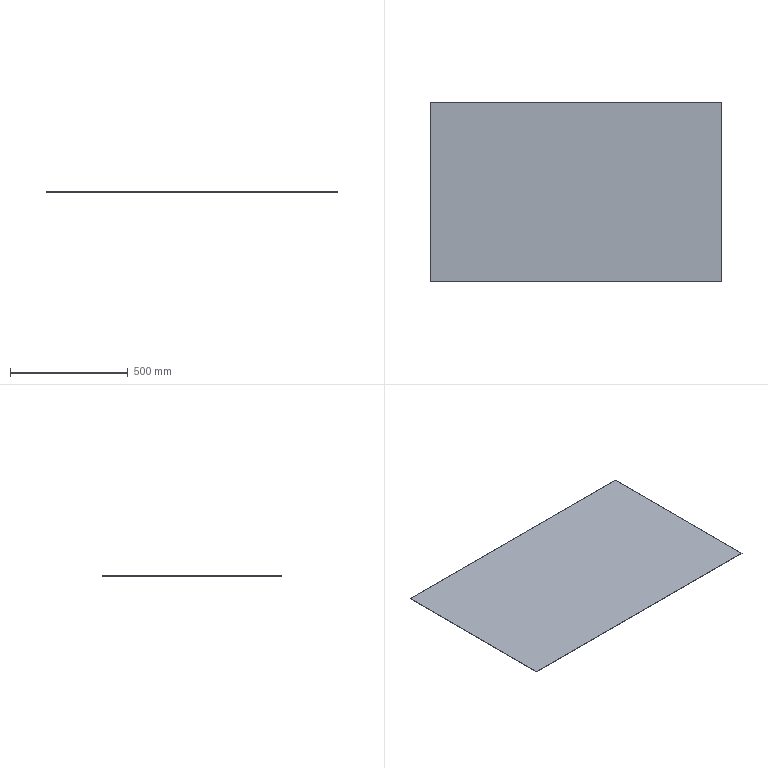Part | SolidWorks | 1 solid | 6 faces | box 1230 x 760 x 1.5 mm | volume 1402200 mm3 | plane 6
STEP:
#1=CARTESIAN_POINT('',(615.,-380.,0.));
#2=VERTEX_POINT('',#1);
#3=CARTESIAN_POINT('',(615.,380.,0.));
#4=VERTEX_POINT('',#3);
#5=CARTESIAN_POINT('',(615.,-380.,0.));
#6=DIRECTION('',(0.,1.,0.));
#7=VECTOR('',#6,1000.);
#8=LINE('',#5,#7);
#9=EDGE_CURVE('',#2,#4,#8,.T.);
#10=ORIENTED_EDGE('',*,*,#9,.T.);
#11=CARTESIAN_POINT('',(615.,380.,1.5));
#12=VERTEX_POINT('',#11);
#13=CARTESIAN_POINT('',(615.,380.,1.5));
#14=DIRECTION('',(0.,0.,-1.));
#15=VECTOR('',#14,1000.);
#16=LINE('',#13,#15);
#17=EDGE_CURVE('',#12,#4,#16,.T.);
#18=ORIENTED_EDGE('',*,*,#17,.F.);
#19=CARTESIAN_POINT('',(615.,-380.,1.5));
#20=VERTEX_POINT('',#19);
#21=CARTESIAN_POINT('',(615.,-380.,1.5));
#22=DIRECTION('',(0.,1.,0.));
#23=VECTOR('',#22,1000.);
#24=LINE('',#21,#23);
#25=EDGE_CURVE('',#20,#12,#24,.T.);
#26=ORIENTED_EDGE('',*,*,#25,.F.);
#27=CARTESIAN_POINT('',(615.,-380.,1.5));
#28=DIRECTION('',(0.,0.,-1.));
#29=VECTOR('',#28,1000.);
#30=LINE('',#27,#29);
#31=EDGE_CURVE('',#20,#2,#30,.T.);
#32=ORIENTED_EDGE('',*,*,#31,.T.);
#33=EDGE_LOOP('',(#10,#18,#26,#32));
#34=FACE_OUTER_BOUND('',#33,.T.);
#35=CARTESIAN_POINT('',(615.,-380.,1.5));
#36=DIRECTION('',(-1.,0.,0.));
#37=DIRECTION('',(0.,0.,1.));
#38=AXIS2_PLACEMENT_3D('',#35,#36,#37);
#39=PLANE('',#38);
#40=ADVANCED_FACE('',(#34),#39,.F.);
#41=CARTESIAN_POINT('',(-615.,380.,0.));
#42=VERTEX_POINT('',#41);
#43=CARTESIAN_POINT('',(615.,380.,0.));
#44=DIRECTION('',(-1.,0.,0.));
#45=VECTOR('',#44,1000.);
#46=LINE('',#43,#45);
#47=EDGE_CURVE('',#4,#42,#46,.T.);
#48=ORIENTED_EDGE('',*,*,#47,.T.);
#49=CARTESIAN_POINT('',(-615.,380.,1.5));
#50=VERTEX_POINT('',#49);
#51=CARTESIAN_POINT('',(-615.,380.,1.5));
#52=DIRECTION('',(0.,0.,-1.));
#53=VECTOR('',#52,1000.);
#54=LINE('',#51,#53);
#55=EDGE_CURVE('',#50,#42,#54,.T.);
#56=ORIENTED_EDGE('',*,*,#55,.F.);
#57=CARTESIAN_POINT('',(615.,380.,1.5));
#58=DIRECTION('',(-1.,0.,0.));
#59=VECTOR('',#58,1000.);
#60=LINE('',#57,#59);
#61=EDGE_CURVE('',#12,#50,#60,.T.);
#62=ORIENTED_EDGE('',*,*,#61,.F.);
#63=ORIENTED_EDGE('',*,*,#17,.T.);
#64=EDGE_LOOP('',(#48,#56,#62,#63));
#65=FACE_OUTER_BOUND('',#64,.T.);
#66=CARTESIAN_POINT('',(615.,380.,1.5));
#67=DIRECTION('',(0.,-1.,0.));
#68=DIRECTION('',(0.,0.,-1.));
#69=AXIS2_PLACEMENT_3D('',#66,#67,#68);
#70=PLANE('',#69);
#71=ADVANCED_FACE('',(#65),#70,.F.);
#72=CARTESIAN_POINT('',(-615.,-380.,0.));
#73=VERTEX_POINT('',#72);
#74=CARTESIAN_POINT('',(-615.,-380.,0.));
#75=DIRECTION('',(0.,-1.,0.));
#76=VECTOR('',#75,1000.);
#77=LINE('',#74,#76);
#78=EDGE_CURVE('',#42,#73,#77,.T.);
#79=ORIENTED_EDGE('',*,*,#78,.T.);
#80=CARTESIAN_POINT('',(-615.,-380.,1.5));
#81=VERTEX_POINT('',#80);
#82=CARTESIAN_POINT('',(-615.,-380.,1.5));
#83=DIRECTION('',(0.,0.,-1.));
#84=VECTOR('',#83,1000.);
#85=LINE('',#82,#84);
#86=EDGE_CURVE('',#81,#73,#85,.T.);
#87=ORIENTED_EDGE('',*,*,#86,.F.);
#88=CARTESIAN_POINT('',(-615.,-380.,1.5));
#89=DIRECTION('',(0.,-1.,0.));
#90=VECTOR('',#89,1000.);
#91=LINE('',#88,#90);
#92=EDGE_CURVE('',#50,#81,#91,.T.);
#93=ORIENTED_EDGE('',*,*,#92,.F.);
#94=ORIENTED_EDGE('',*,*,#55,.T.);
#95=EDGE_LOOP('',(#79,#87,#93,#94));
#96=FACE_OUTER_BOUND('',#95,.T.);
#97=CARTESIAN_POINT('',(-615.,-380.,1.5));
#98=DIRECTION('',(1.,0.,0.));
#99=DIRECTION('',(0.,0.,-1.));
#100=AXIS2_PLACEMENT_3D('',#97,#98,#99);
#101=PLANE('',#100);
#102=ADVANCED_FACE('',(#96),#101,.F.);
#103=CARTESIAN_POINT('',(615.,-380.,0.));
#104=DIRECTION('',(1.,0.,0.));
#105=VECTOR('',#104,1000.);
#106=LINE('',#103,#105);
#107=EDGE_CURVE('',#73,#2,#106,.T.);
#108=ORIENTED_EDGE('',*,*,#107,.T.);
#109=ORIENTED_EDGE('',*,*,#31,.F.);
#110=CARTESIAN_POINT('',(615.,-380.,1.5));
#111=DIRECTION('',(1.,0.,0.));
#112=VECTOR('',#111,1000.);
#113=LINE('',#110,#112);
#114=EDGE_CURVE('',#81,#20,#113,.T.);
#115=ORIENTED_EDGE('',*,*,#114,.F.);
#116=ORIENTED_EDGE('',*,*,#86,.T.);
#117=EDGE_LOOP('',(#108,#109,#115,#116));
#118=FACE_OUTER_BOUND('',#117,.T.);
#119=CARTESIAN_POINT('',(615.,-380.,1.5));
#120=DIRECTION('',(0.,1.,0.));
#121=DIRECTION('',(0.,0.,1.));
#122=AXIS2_PLACEMENT_3D('',#119,#120,#121);
#123=PLANE('',#122);
#124=ADVANCED_FACE('',(#118),#123,.F.);
#125=ORIENTED_EDGE('',*,*,#25,.T.);
#126=ORIENTED_EDGE('',*,*,#61,.T.);
#127=ORIENTED_EDGE('',*,*,#92,.T.);
#128=ORIENTED_EDGE('',*,*,#114,.T.);
#129=EDGE_LOOP('',(#125,#126,#127,#128));
#130=FACE_OUTER_BOUND('',#129,.T.);
#131=CARTESIAN_POINT('',(0.,0.,1.5));
#132=DIRECTION('',(0.,0.,1.));
#133=DIRECTION('',(1.,0.,0.));
#134=AXIS2_PLACEMENT_3D('',#131,#132,#133);
#135=PLANE('',#134);
#136=ADVANCED_FACE('',(#130),#135,.T.);
#137=ORIENTED_EDGE('',*,*,#9,.F.);
#138=ORIENTED_EDGE('',*,*,#107,.F.);
#139=ORIENTED_EDGE('',*,*,#78,.F.);
#140=ORIENTED_EDGE('',*,*,#47,.F.);
#141=EDGE_LOOP('',(#137,#138,#139,#140));
#142=FACE_OUTER_BOUND('',#141,.T.);
#143=CARTESIAN_POINT('',(0.,0.,0.));
#144=DIRECTION('',(0.,0.,1.));
#145=DIRECTION('',(1.,0.,0.));
#146=AXIS2_PLACEMENT_3D('',#143,#144,#145);
#147=PLANE('',#146);
#148=ADVANCED_FACE('',(#142),#147,.F.);
#149=CLOSED_SHELL('',(#40,#71,#102,#124,#136,#148));
#150=MANIFOLD_SOLID_BREP('',#149);
#151=CARTESIAN_POINT('',(0.,0.,0.));
#152=DIRECTION('',(0.,0.,1.));
#153=DIRECTION('',(1.,0.,0.));
#154=AXIS2_PLACEMENT_3D('',#151,#152,#153);
#155=(LENGTH_UNIT()NAMED_UNIT(*)SI_UNIT(.MILLI.,.METRE.));
#156=UNCERTAINTY_MEASURE_WITH_UNIT(LENGTH_MEASURE(0.00001),#155,'','');
#157=(NAMED_UNIT(*)PLANE_ANGLE_UNIT()SI_UNIT($,.RADIAN.));
#158=(NAMED_UNIT(*)SI_UNIT($,.STERADIAN.)SOLID_ANGLE_UNIT());
#159=(GEOMETRIC_REPRESENTATION_CONTEXT(3)GLOBAL_UNCERTAINTY_ASSIGNED_CONTEXT((#156))GLOBAL_UNIT_ASSIGNED_CONTEXT((#155,#157,#158))REPRESENTATION_CONTEXT('',''));
#160=ADVANCED_BREP_SHAPE_REPRESENTATION('',(#150,#154),#159);